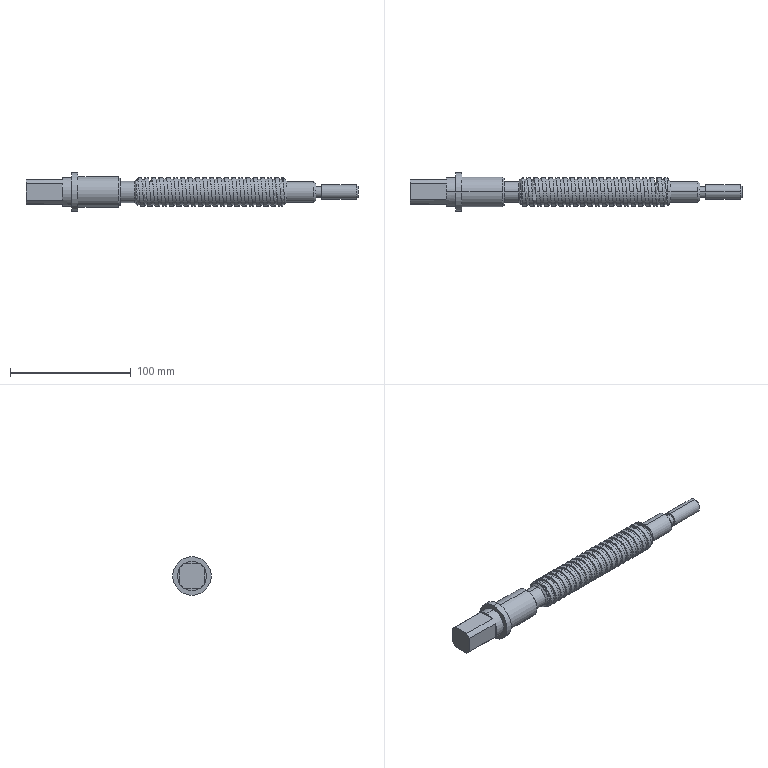Part | SolidWorks | features Chamfer 2, ICE 2, Helix 1, Revolution 1, SweepCut 1 | 1 solid | 87 faces | box 275 x 32 x 32 mm | volume 98035 mm3 | cylinder 56 | plane 17 | cone 11 | spline 3 | commonest cylinder face diameters 24 x44 9 x2 12 x2 17 x2 17.5 x2 25 x2